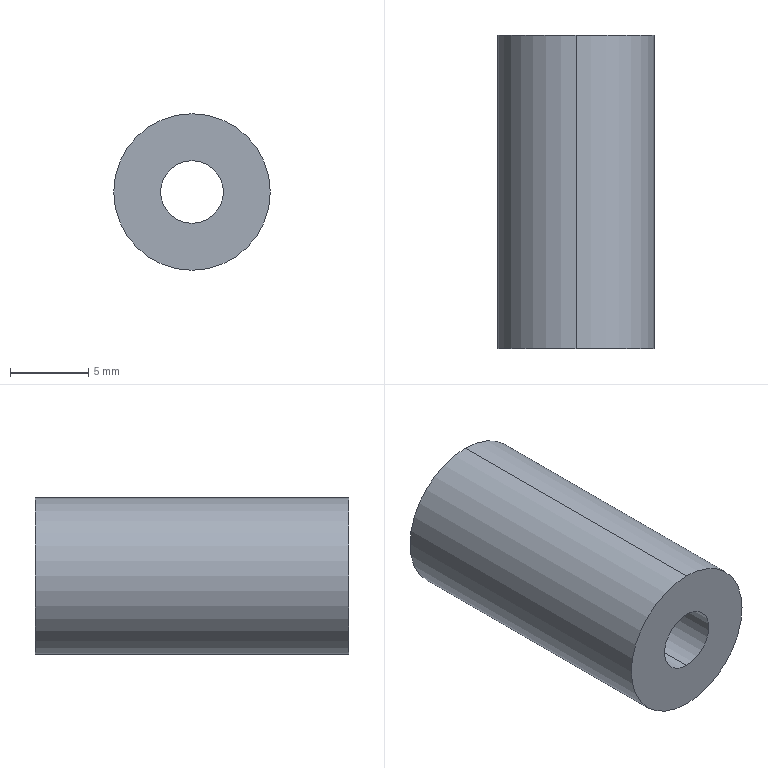Part | SolidWorks | features BaseBody 1 | 1 solid | 6 faces | box 10 x 20 x 10 mm | volume 1319 mm3 | cylinder 4 | plane 2 | commonest cylinder face diameters 4 x2 10 x2
STEP:
#1=CARTESIAN_POINT('',(0.,10.,-5.));
#2=VERTEX_POINT('',#1);
#3=CARTESIAN_POINT('',(0.,10.,5.));
#4=VERTEX_POINT('',#3);
#5=CARTESIAN_POINT('',(0.,10.,0.));
#6=DIRECTION('',(0.,-1.,0.));
#7=DIRECTION('',(0.,0.,-1.));
#8=AXIS2_PLACEMENT_3D('',#5,#6,#7);
#9=CIRCLE('',#8,5.);
#10=EDGE_CURVE('',#2,#4,#9,.T.);
#11=ORIENTED_EDGE('',*,*,#10,.T.);
#12=CARTESIAN_POINT('',(0.,-10.,5.));
#13=VERTEX_POINT('',#12);
#14=CARTESIAN_POINT('',(0.,10.,5.));
#15=DIRECTION('',(0.,-1.,0.));
#16=VECTOR('',#15,1000.);
#17=LINE('',#14,#16);
#18=EDGE_CURVE('',#4,#13,#17,.T.);
#19=ORIENTED_EDGE('',*,*,#18,.T.);
#20=CARTESIAN_POINT('',(0.,-10.,-5.));
#21=VERTEX_POINT('',#20);
#22=CARTESIAN_POINT('',(0.,-10.,0.));
#23=DIRECTION('',(0.,1.,0.));
#24=DIRECTION('',(0.,0.,-1.));
#25=AXIS2_PLACEMENT_3D('',#22,#23,#24);
#26=CIRCLE('',#25,5.);
#27=EDGE_CURVE('',#13,#21,#26,.T.);
#28=ORIENTED_EDGE('',*,*,#27,.T.);
#29=CARTESIAN_POINT('',(0.,10.,-5.));
#30=DIRECTION('',(0.,-1.,0.));
#31=VECTOR('',#30,1000.);
#32=LINE('',#29,#31);
#33=EDGE_CURVE('',#2,#21,#32,.T.);
#34=ORIENTED_EDGE('',*,*,#33,.F.);
#35=EDGE_LOOP('',(#11,#19,#28,#34));
#36=FACE_OUTER_BOUND('',#35,.T.);
#37=CARTESIAN_POINT('',(0.,10.,0.));
#38=DIRECTION('',(0.,-1.,0.));
#39=DIRECTION('',(0.,0.,-1.));
#40=AXIS2_PLACEMENT_3D('',#37,#38,#39);
#41=CYLINDRICAL_SURFACE('',#40,5.);
#42=ADVANCED_FACE('',(#36),#41,.T.);
#43=CARTESIAN_POINT('',(0.,10.,2.));
#44=VERTEX_POINT('',#43);
#45=CARTESIAN_POINT('',(0.,10.,-2.));
#46=VERTEX_POINT('',#45);
#47=CARTESIAN_POINT('',(0.,10.,0.));
#48=DIRECTION('',(0.,-1.,0.));
#49=DIRECTION('',(0.,0.,-1.));
#50=AXIS2_PLACEMENT_3D('',#47,#48,#49);
#51=CIRCLE('',#50,2.);
#52=EDGE_CURVE('',#44,#46,#51,.T.);
#53=ORIENTED_EDGE('',*,*,#52,.F.);
#54=CARTESIAN_POINT('',(0.,-10.,2.));
#55=VERTEX_POINT('',#54);
#56=CARTESIAN_POINT('',(0.,10.,2.));
#57=DIRECTION('',(0.,-1.,0.));
#58=VECTOR('',#57,1000.);
#59=LINE('',#56,#58);
#60=EDGE_CURVE('',#44,#55,#59,.T.);
#61=ORIENTED_EDGE('',*,*,#60,.T.);
#62=CARTESIAN_POINT('',(0.,-10.,-2.));
#63=VERTEX_POINT('',#62);
#64=CARTESIAN_POINT('',(0.,-10.,0.));
#65=DIRECTION('',(0.,-1.,0.));
#66=DIRECTION('',(0.,0.,-1.));
#67=AXIS2_PLACEMENT_3D('',#64,#65,#66);
#68=CIRCLE('',#67,2.);
#69=EDGE_CURVE('',#55,#63,#68,.T.);
#70=ORIENTED_EDGE('',*,*,#69,.T.);
#71=CARTESIAN_POINT('',(0.,10.,-2.));
#72=DIRECTION('',(0.,-1.,0.));
#73=VECTOR('',#72,1000.);
#74=LINE('',#71,#73);
#75=EDGE_CURVE('',#46,#63,#74,.T.);
#76=ORIENTED_EDGE('',*,*,#75,.F.);
#77=EDGE_LOOP('',(#53,#61,#70,#76));
#78=FACE_OUTER_BOUND('',#77,.T.);
#79=CARTESIAN_POINT('',(0.,10.,0.));
#80=DIRECTION('',(0.,-1.,0.));
#81=DIRECTION('',(0.,0.,-1.));
#82=AXIS2_PLACEMENT_3D('',#79,#80,#81);
#83=CYLINDRICAL_SURFACE('',#82,2.);
#84=ADVANCED_FACE('',(#78),#83,.F.);
#85=ORIENTED_EDGE('',*,*,#18,.F.);
#86=CARTESIAN_POINT('',(0.,10.,0.));
#87=DIRECTION('',(0.,-1.,0.));
#88=DIRECTION('',(0.,0.,-1.));
#89=AXIS2_PLACEMENT_3D('',#86,#87,#88);
#90=CIRCLE('',#89,5.);
#91=EDGE_CURVE('',#4,#2,#90,.T.);
#92=ORIENTED_EDGE('',*,*,#91,.T.);
#93=ORIENTED_EDGE('',*,*,#33,.T.);
#94=CARTESIAN_POINT('',(0.,-10.,0.));
#95=DIRECTION('',(0.,1.,0.));
#96=DIRECTION('',(0.,0.,-1.));
#97=AXIS2_PLACEMENT_3D('',#94,#95,#96);
#98=CIRCLE('',#97,5.);
#99=EDGE_CURVE('',#21,#13,#98,.T.);
#100=ORIENTED_EDGE('',*,*,#99,.T.);
#101=EDGE_LOOP('',(#85,#92,#93,#100));
#102=FACE_OUTER_BOUND('',#101,.T.);
#103=CARTESIAN_POINT('',(0.,10.,0.));
#104=DIRECTION('',(0.,-1.,0.));
#105=DIRECTION('',(0.,0.,-1.));
#106=AXIS2_PLACEMENT_3D('',#103,#104,#105);
#107=CYLINDRICAL_SURFACE('',#106,5.);
#108=ADVANCED_FACE('',(#102),#107,.T.);
#109=CARTESIAN_POINT('',(0.,-10.,0.));
#110=DIRECTION('',(0.,-1.,0.));
#111=DIRECTION('',(0.,0.,-1.));
#112=AXIS2_PLACEMENT_3D('',#109,#110,#111);
#113=CIRCLE('',#112,2.);
#114=EDGE_CURVE('',#63,#55,#113,.T.);
#115=ORIENTED_EDGE('',*,*,#114,.F.);
#116=ORIENTED_EDGE('',*,*,#69,.F.);
#117=EDGE_LOOP('',(#115,#116));
#118=FACE_BOUND('',#117,.T.);
#119=ORIENTED_EDGE('',*,*,#99,.F.);
#120=ORIENTED_EDGE('',*,*,#27,.F.);
#121=EDGE_LOOP('',(#119,#120));
#122=FACE_OUTER_BOUND('',#121,.T.);
#123=CARTESIAN_POINT('',(0.,-10.,0.));
#124=DIRECTION('',(0.,1.,0.));
#125=DIRECTION('',(0.,0.,1.));
#126=AXIS2_PLACEMENT_3D('',#123,#124,#125);
#127=PLANE('',#126);
#128=ADVANCED_FACE('',(#118,#122),#127,.F.);
#129=CARTESIAN_POINT('',(0.,10.,0.));
#130=DIRECTION('',(0.,-1.,0.));
#131=DIRECTION('',(0.,0.,-1.));
#132=AXIS2_PLACEMENT_3D('',#129,#130,#131);
#133=CIRCLE('',#132,2.);
#134=EDGE_CURVE('',#46,#44,#133,.T.);
#135=ORIENTED_EDGE('',*,*,#134,.T.);
#136=ORIENTED_EDGE('',*,*,#52,.T.);
#137=EDGE_LOOP('',(#135,#136));
#138=FACE_BOUND('',#137,.T.);
#139=ORIENTED_EDGE('',*,*,#10,.F.);
#140=ORIENTED_EDGE('',*,*,#91,.F.);
#141=EDGE_LOOP('',(#139,#140));
#142=FACE_OUTER_BOUND('',#141,.T.);
#143=CARTESIAN_POINT('',(0.,10.,0.));
#144=DIRECTION('',(0.,1.,0.));
#145=DIRECTION('',(0.,0.,1.));
#146=AXIS2_PLACEMENT_3D('',#143,#144,#145);
#147=PLANE('',#146);
#148=ADVANCED_FACE('',(#138,#142),#147,.T.);
#149=ORIENTED_EDGE('',*,*,#60,.F.);
#150=ORIENTED_EDGE('',*,*,#134,.F.);
#151=ORIENTED_EDGE('',*,*,#75,.T.);
#152=ORIENTED_EDGE('',*,*,#114,.T.);
#153=EDGE_LOOP('',(#149,#150,#151,#152));
#154=FACE_OUTER_BOUND('',#153,.T.);
#155=CARTESIAN_POINT('',(0.,10.,0.));
#156=DIRECTION('',(0.,-1.,0.));
#157=DIRECTION('',(0.,0.,-1.));
#158=AXIS2_PLACEMENT_3D('',#155,#156,#157);
#159=CYLINDRICAL_SURFACE('',#158,2.);
#160=ADVANCED_FACE('',(#154),#159,.F.);
#161=CLOSED_SHELL('',(#42,#84,#108,#128,#148,#160));
#162=MANIFOLD_SOLID_BREP('',#161);
#163=CARTESIAN_POINT('',(0.,0.,0.));
#164=DIRECTION('',(0.,0.,1.));
#165=DIRECTION('',(1.,0.,0.));
#166=AXIS2_PLACEMENT_3D('',#163,#164,#165);
#167=(LENGTH_UNIT()NAMED_UNIT(*)SI_UNIT(.MILLI.,.METRE.));
#168=UNCERTAINTY_MEASURE_WITH_UNIT(LENGTH_MEASURE(0.00001),#167,'','');
#169=(NAMED_UNIT(*)PLANE_ANGLE_UNIT()SI_UNIT($,.RADIAN.));
#170=(NAMED_UNIT(*)SI_UNIT($,.STERADIAN.)SOLID_ANGLE_UNIT());
#171=(GEOMETRIC_REPRESENTATION_CONTEXT(3)GLOBAL_UNCERTAINTY_ASSIGNED_CONTEXT((#168))GLOBAL_UNIT_ASSIGNED_CONTEXT((#167,#169,#170))REPRESENTATION_CONTEXT('',''));
#172=ADVANCED_BREP_SHAPE_REPRESENTATION('',(#162,#166),#171);